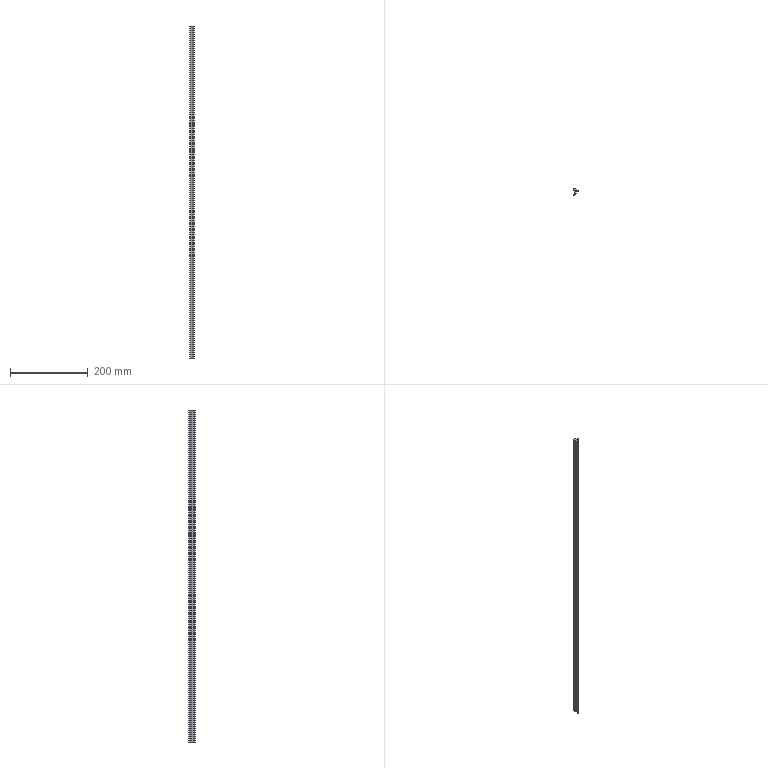Part | SolidWorks | features BaseBody 1, MoveFace 1 | 1 solid | 20 faces | box 10.8 x 17.5 x 856 mm | volume 67453 mm3 | cylinder 11 | plane 9 | commonest cylinder face diameters 1.6 x2 14 x2 0.4 x1 0.6 x1 0.8 x1 2.6 x1
STEP:
#1=CARTESIAN_POINT('',(-3.236,-11.055,756.));
#2=VERTEX_POINT('',#1);
#3=CARTESIAN_POINT('',(-4.3,-10.3,756.));
#4=VERTEX_POINT('',#3);
#5=CARTESIAN_POINT('',(-3.5,-10.3,756.));
#6=DIRECTION('',(0.,0.,-1.));
#7=DIRECTION('',(1.,0.,0.));
#8=AXIS2_PLACEMENT_3D('',#5,#6,#7);
#9=CIRCLE('',#8,0.8);
#10=EDGE_CURVE('',#2,#4,#9,.T.);
#11=ORIENTED_EDGE('',*,*,#10,.T.);
#12=CARTESIAN_POINT('',(-4.3,-10.3,-100.));
#13=VERTEX_POINT('',#12);
#14=CARTESIAN_POINT('',(-4.3,-10.3,-100.));
#15=DIRECTION('',(0.,0.,-1.));
#16=VECTOR('',#15,1000.);
#17=LINE('',#14,#16);
#18=EDGE_CURVE('',#4,#13,#17,.T.);
#19=ORIENTED_EDGE('',*,*,#18,.T.);
#20=CARTESIAN_POINT('',(-3.236,-11.055,-100.));
#21=VERTEX_POINT('',#20);
#22=CARTESIAN_POINT('',(-3.5,-10.3,-100.));
#23=DIRECTION('',(0.,0.,1.));
#24=DIRECTION('',(-1.,0.,0.));
#25=AXIS2_PLACEMENT_3D('',#22,#23,#24);
#26=CIRCLE('',#25,0.8);
#27=EDGE_CURVE('',#13,#21,#26,.T.);
#28=ORIENTED_EDGE('',*,*,#27,.T.);
#29=CARTESIAN_POINT('',(-3.236,-11.055,-100.));
#30=DIRECTION('',(0.,0.,-1.));
#31=VECTOR('',#30,1000.);
#32=LINE('',#29,#31);
#33=EDGE_CURVE('',#2,#21,#32,.T.);
#34=ORIENTED_EDGE('',*,*,#33,.F.);
#35=EDGE_LOOP('',(#11,#19,#28,#34));
#36=FACE_OUTER_BOUND('',#35,.T.);
#37=CARTESIAN_POINT('',(-3.5,-10.3,-100.));
#38=DIRECTION('',(0.,0.,-1.));
#39=DIRECTION('',(-1.,0.,0.));
#40=AXIS2_PLACEMENT_3D('',#37,#38,#39);
#41=CYLINDRICAL_SURFACE('',#40,0.8);
#42=ADVANCED_FACE('',(#36),#41,.T.);
#43=CARTESIAN_POINT('',(1.184,-6.397,-100.));
#44=VERTEX_POINT('',#43);
#45=CARTESIAN_POINT('',(-5.702,-4.29,-100.));
#46=DIRECTION('',(0.,0.,1.));
#47=DIRECTION('',(-1.,0.,0.));
#48=AXIS2_PLACEMENT_3D('',#45,#46,#47);
#49=CIRCLE('',#48,7.201);
#50=EDGE_CURVE('',#21,#44,#49,.T.);
#51=ORIENTED_EDGE('',*,*,#50,.T.);
#52=CARTESIAN_POINT('',(1.184,-6.397,756.));
#53=VERTEX_POINT('',#52);
#54=CARTESIAN_POINT('',(1.184,-6.397,-100.));
#55=DIRECTION('',(0.,0.,1.));
#56=VECTOR('',#55,1000.);
#57=LINE('',#54,#56);
#58=EDGE_CURVE('',#44,#53,#57,.T.);
#59=ORIENTED_EDGE('',*,*,#58,.T.);
#60=CARTESIAN_POINT('',(-5.702,-4.29,756.));
#61=DIRECTION('',(0.,0.,-1.));
#62=DIRECTION('',(1.,0.,0.));
#63=AXIS2_PLACEMENT_3D('',#60,#61,#62);
#64=CIRCLE('',#63,7.201);
#65=EDGE_CURVE('',#53,#2,#64,.T.);
#66=ORIENTED_EDGE('',*,*,#65,.T.);
#67=ORIENTED_EDGE('',*,*,#33,.T.);
#68=EDGE_LOOP('',(#51,#59,#66,#67));
#69=FACE_OUTER_BOUND('',#68,.T.);
#70=CARTESIAN_POINT('',(-5.702,-4.29,-100.));
#71=DIRECTION('',(0.,0.,-1.));
#72=DIRECTION('',(-1.,0.,0.));
#73=AXIS2_PLACEMENT_3D('',#70,#71,#72);
#74=CYLINDRICAL_SURFACE('',#73,7.201);
#75=ADVANCED_FACE('',(#69),#74,.T.);
#76=CARTESIAN_POINT('',(0.9,-6.,-100.));
#77=VERTEX_POINT('',#76);
#78=CARTESIAN_POINT('',(0.9,-6.3,-100.));
#79=DIRECTION('',(0.,0.,1.));
#80=DIRECTION('',(-1.,0.,0.));
#81=AXIS2_PLACEMENT_3D('',#78,#79,#80);
#82=CIRCLE('',#81,0.3);
#83=EDGE_CURVE('',#44,#77,#82,.T.);
#84=ORIENTED_EDGE('',*,*,#83,.T.);
#85=CARTESIAN_POINT('',(0.9,-6.,756.));
#86=VERTEX_POINT('',#85);
#87=CARTESIAN_POINT('',(0.9,-6.,-100.));
#88=DIRECTION('',(0.,0.,1.));
#89=VECTOR('',#88,1000.);
#90=LINE('',#87,#89);
#91=EDGE_CURVE('',#77,#86,#90,.T.);
#92=ORIENTED_EDGE('',*,*,#91,.T.);
#93=CARTESIAN_POINT('',(0.9,-6.3,756.));
#94=DIRECTION('',(0.,0.,-1.));
#95=DIRECTION('',(1.,0.,0.));
#96=AXIS2_PLACEMENT_3D('',#93,#94,#95);
#97=CIRCLE('',#96,0.3);
#98=EDGE_CURVE('',#86,#53,#97,.T.);
#99=ORIENTED_EDGE('',*,*,#98,.T.);
#100=ORIENTED_EDGE('',*,*,#58,.F.);
#101=EDGE_LOOP('',(#84,#92,#99,#100));
#102=FACE_OUTER_BOUND('',#101,.T.);
#103=CARTESIAN_POINT('',(0.9,-6.3,-100.));
#104=DIRECTION('',(0.,0.,-1.));
#105=DIRECTION('',(-1.,0.,0.));
#106=AXIS2_PLACEMENT_3D('',#103,#104,#105);
#107=CYLINDRICAL_SURFACE('',#106,0.3);
#108=ADVANCED_FACE('',(#102),#107,.T.);
#109=CARTESIAN_POINT('',(-2.5,-0.5,-100.));
#110=VERTEX_POINT('',#109);
#111=CARTESIAN_POINT('',(-2.5,-6.153,-100.));
#112=VERTEX_POINT('',#111);
#113=CARTESIAN_POINT('',(-2.5,-6.397,-100.));
#114=DIRECTION('',(0.,-1.,0.));
#115=VECTOR('',#114,1000.);
#116=LINE('',#113,#115);
#117=EDGE_CURVE('',#110,#112,#116,.T.);
#118=ORIENTED_EDGE('',*,*,#117,.F.);
#119=CARTESIAN_POINT('',(-4.2,1.695,-100.));
#120=VERTEX_POINT('',#119);
#121=CARTESIAN_POINT('',(-1.701,1.875,-100.));
#122=DIRECTION('',(0.,0.,1.));
#123=DIRECTION('',(-1.,0.,0.));
#124=AXIS2_PLACEMENT_3D('',#121,#122,#123);
#125=CIRCLE('',#124,2.506);
#126=EDGE_CURVE('',#120,#110,#125,.T.);
#127=ORIENTED_EDGE('',*,*,#126,.F.);
#128=CARTESIAN_POINT('',(-4.2,5.1,-100.));
#129=VERTEX_POINT('',#128);
#130=CARTESIAN_POINT('',(-4.2,-6.397,-100.));
#131=DIRECTION('',(0.,-1.,0.));
#132=VECTOR('',#131,1000.);
#133=LINE('',#130,#132);
#134=EDGE_CURVE('',#129,#120,#133,.T.);
#135=ORIENTED_EDGE('',*,*,#134,.F.);
#136=CARTESIAN_POINT('',(-2.892,6.4,-100.));
#137=VERTEX_POINT('',#136);
#138=CARTESIAN_POINT('',(-2.9,5.1,-100.));
#139=DIRECTION('',(0.,0.,1.));
#140=DIRECTION('',(-1.,0.,0.));
#141=AXIS2_PLACEMENT_3D('',#138,#139,#140);
#142=CIRCLE('',#141,1.3);
#143=EDGE_CURVE('',#137,#129,#142,.T.);
#144=ORIENTED_EDGE('',*,*,#143,.F.);
#145=CARTESIAN_POINT('',(0.5,5.5,-100.));
#146=VERTEX_POINT('',#145);
#147=CARTESIAN_POINT('',(-2.934,-0.5999,-100.));
#148=DIRECTION('',(0.,0.,1.));
#149=DIRECTION('',(-1.,0.,0.));
#150=AXIS2_PLACEMENT_3D('',#147,#148,#149);
#151=CIRCLE('',#150,7.);
#152=EDGE_CURVE('',#146,#137,#151,.T.);
#153=ORIENTED_EDGE('',*,*,#152,.F.);
#154=CARTESIAN_POINT('',(5.5,1.7,-100.));
#155=VERTEX_POINT('',#154);
#156=CARTESIAN_POINT('',(5.5,1.7,-100.));
#157=DIRECTION('',(-0.7962,0.6051,0.));
#158=VECTOR('',#157,1000.);
#159=LINE('',#156,#158);
#160=EDGE_CURVE('',#155,#146,#159,.T.);
#161=ORIENTED_EDGE('',*,*,#160,.F.);
#162=CARTESIAN_POINT('',(6.458,-0.2215,-100.));
#163=VERTEX_POINT('',#162);
#164=CARTESIAN_POINT('',(6.458,-0.2215,-100.));
#165=DIRECTION('',(-0.4462,0.8949,0.));
#166=VECTOR('',#165,1000.);
#167=LINE('',#164,#166);
#168=EDGE_CURVE('',#163,#155,#167,.T.);
#169=ORIENTED_EDGE('',*,*,#168,.F.);
#170=CARTESIAN_POINT('',(5.895,-0.7433,-100.));
#171=VERTEX_POINT('',#170);
#172=CARTESIAN_POINT('',(6.1,-0.4,-100.));
#173=DIRECTION('',(0.,0.,1.));
#174=DIRECTION('',(-1.,0.,0.));
#175=AXIS2_PLACEMENT_3D('',#172,#173,#174);
#176=CIRCLE('',#175,0.4);
#177=EDGE_CURVE('',#171,#163,#176,.T.);
#178=ORIENTED_EDGE('',*,*,#177,.F.);
#179=CARTESIAN_POINT('',(3.,0.,-100.));
#180=VERTEX_POINT('',#179);
#181=CARTESIAN_POINT('',(2.746,-6.995,-100.));
#182=DIRECTION('',(0.,0.,-1.));
#183=DIRECTION('',(-1.,0.,0.));
#184=AXIS2_PLACEMENT_3D('',#181,#182,#183);
#185=CIRCLE('',#184,7.);
#186=EDGE_CURVE('',#180,#171,#185,.T.);
#187=ORIENTED_EDGE('',*,*,#186,.F.);
#188=CARTESIAN_POINT('',(0.,0.,-100.));
#189=VERTEX_POINT('',#188);
#190=CARTESIAN_POINT('',(-6.814,0.,-100.));
#191=DIRECTION('',(1.,0.,0.));
#192=VECTOR('',#191,1000.);
#193=LINE('',#190,#192);
#194=EDGE_CURVE('',#189,#180,#193,.T.);
#195=ORIENTED_EDGE('',*,*,#194,.F.);
#196=CARTESIAN_POINT('',(0.,-5.8,-100.));
#197=VERTEX_POINT('',#196);
#198=CARTESIAN_POINT('',(0.,-6.397,-100.));
#199=DIRECTION('',(0.,1.,0.));
#200=VECTOR('',#199,1000.);
#201=LINE('',#198,#200);
#202=EDGE_CURVE('',#197,#189,#201,.T.);
#203=ORIENTED_EDGE('',*,*,#202,.F.);
#204=CARTESIAN_POINT('',(0.2,-6.,-100.));
#205=VERTEX_POINT('',#204);
#206=CARTESIAN_POINT('',(0.2,-5.8,-100.));
#207=DIRECTION('',(0.,0.,1.));
#208=DIRECTION('',(-1.,0.,0.));
#209=AXIS2_PLACEMENT_3D('',#206,#207,#208);
#210=CIRCLE('',#209,0.2);
#211=EDGE_CURVE('',#197,#205,#210,.T.);
#212=ORIENTED_EDGE('',*,*,#211,.T.);
#213=CARTESIAN_POINT('',(-6.814,-6.,-100.));
#214=DIRECTION('',(-1.,0.,0.));
#215=VECTOR('',#214,1000.);
#216=LINE('',#213,#215);
#217=EDGE_CURVE('',#77,#205,#216,.T.);
#218=ORIENTED_EDGE('',*,*,#217,.F.);
#219=ORIENTED_EDGE('',*,*,#83,.F.);
#220=ORIENTED_EDGE('',*,*,#50,.F.);
#221=ORIENTED_EDGE('',*,*,#27,.F.);
#222=CARTESIAN_POINT('',(-3.998,-9.674,-100.));
#223=VERTEX_POINT('',#222);
#224=CARTESIAN_POINT('',(-3.5,-10.3,-100.));
#225=DIRECTION('',(0.,0.,1.));
#226=DIRECTION('',(-1.,0.,0.));
#227=AXIS2_PLACEMENT_3D('',#224,#225,#226);
#228=CIRCLE('',#227,0.8);
#229=EDGE_CURVE('',#223,#13,#228,.T.);
#230=ORIENTED_EDGE('',*,*,#229,.F.);
#231=CARTESIAN_POINT('',(-6.814,-6.397,-100.));
#232=DIRECTION('',(0.,0.,-1.));
#233=DIRECTION('',(-1.,0.,0.));
#234=AXIS2_PLACEMENT_3D('',#231,#232,#233);
#235=CIRCLE('',#234,4.321);
#236=EDGE_CURVE('',#112,#223,#235,.T.);
#237=ORIENTED_EDGE('',*,*,#236,.F.);
#238=EDGE_LOOP('',(#118,#127,#135,#144,#153,#161,#169,#178,#187,#195,#203,#212,#218,#219,#220,#221,#230,#237));
#239=FACE_OUTER_BOUND('',#238,.T.);
#240=CARTESIAN_POINT('',(-6.814,-6.397,-100.));
#241=DIRECTION('',(0.,0.,1.));
#242=DIRECTION('',(1.,0.,0.));
#243=AXIS2_PLACEMENT_3D('',#240,#241,#242);
#244=PLANE('',#243);
#245=ADVANCED_FACE('',(#239),#244,.F.);
#246=ORIENTED_EDGE('',*,*,#18,.F.);
#247=CARTESIAN_POINT('',(-3.998,-9.674,756.));
#248=VERTEX_POINT('',#247);
#249=CARTESIAN_POINT('',(-3.5,-10.3,756.));
#250=DIRECTION('',(0.,0.,-1.));
#251=DIRECTION('',(1.,0.,0.));
#252=AXIS2_PLACEMENT_3D('',#249,#250,#251);
#253=CIRCLE('',#252,0.8);
#254=EDGE_CURVE('',#4,#248,#253,.T.);
#255=ORIENTED_EDGE('',*,*,#254,.T.);
#256=CARTESIAN_POINT('',(-3.998,-9.674,-100.));
#257=DIRECTION('',(0.,0.,-1.));
#258=VECTOR('',#257,1000.);
#259=LINE('',#256,#258);
#260=EDGE_CURVE('',#248,#223,#259,.T.);
#261=ORIENTED_EDGE('',*,*,#260,.T.);
#262=ORIENTED_EDGE('',*,*,#229,.T.);
#263=EDGE_LOOP('',(#246,#255,#261,#262));
#264=FACE_OUTER_BOUND('',#263,.T.);
#265=CARTESIAN_POINT('',(-3.5,-10.3,-100.));
#266=DIRECTION('',(0.,0.,-1.));
#267=DIRECTION('',(-1.,0.,0.));
#268=AXIS2_PLACEMENT_3D('',#265,#266,#267);
#269=CYLINDRICAL_SURFACE('',#268,0.8);
#270=ADVANCED_FACE('',(#264),#269,.T.);
#271=CARTESIAN_POINT('',(-4.2,1.695,756.));
#272=VERTEX_POINT('',#271);
#273=CARTESIAN_POINT('',(-2.5,-0.5,756.));
#274=VERTEX_POINT('',#273);
#275=CARTESIAN_POINT('',(-1.701,1.875,756.));
#276=DIRECTION('',(0.,0.,1.));
#277=DIRECTION('',(1.,0.,0.));
#278=AXIS2_PLACEMENT_3D('',#275,#276,#277);
#279=CIRCLE('',#278,2.506);
#280=EDGE_CURVE('',#272,#274,#279,.T.);
#281=ORIENTED_EDGE('',*,*,#280,.T.);
#282=CARTESIAN_POINT('',(-2.5,-6.153,756.));
#283=VERTEX_POINT('',#282);
#284=CARTESIAN_POINT('',(-2.5,-6.397,756.));
#285=DIRECTION('',(0.,-1.,0.));
#286=VECTOR('',#285,1000.);
#287=LINE('',#284,#286);
#288=EDGE_CURVE('',#274,#283,#287,.T.);
#289=ORIENTED_EDGE('',*,*,#288,.T.);
#290=CARTESIAN_POINT('',(-6.814,-6.397,756.));
#291=DIRECTION('',(0.,0.,-1.));
#292=DIRECTION('',(1.,0.,0.));
#293=AXIS2_PLACEMENT_3D('',#290,#291,#292);
#294=CIRCLE('',#293,4.321);
#295=EDGE_CURVE('',#283,#248,#294,.T.);
#296=ORIENTED_EDGE('',*,*,#295,.T.);
#297=ORIENTED_EDGE('',*,*,#254,.F.);
#298=ORIENTED_EDGE('',*,*,#10,.F.);
#299=ORIENTED_EDGE('',*,*,#65,.F.);
#300=ORIENTED_EDGE('',*,*,#98,.F.);
#301=CARTESIAN_POINT('',(0.2,-6.,756.));
#302=VERTEX_POINT('',#301);
#303=CARTESIAN_POINT('',(-6.814,-6.,756.));
#304=DIRECTION('',(-1.,0.,0.));
#305=VECTOR('',#304,1000.);
#306=LINE('',#303,#305);
#307=EDGE_CURVE('',#86,#302,#306,.T.);
#308=ORIENTED_EDGE('',*,*,#307,.T.);
#309=CARTESIAN_POINT('',(0.,-5.8,756.));
#310=VERTEX_POINT('',#309);
#311=CARTESIAN_POINT('',(0.2,-5.8,756.));
#312=DIRECTION('',(0.,0.,-1.));
#313=DIRECTION('',(1.,0.,0.));
#314=AXIS2_PLACEMENT_3D('',#311,#312,#313);
#315=CIRCLE('',#314,0.2);
#316=EDGE_CURVE('',#302,#310,#315,.T.);
#317=ORIENTED_EDGE('',*,*,#316,.T.);
#318=CARTESIAN_POINT('',(0.,0.,756.));
#319=VERTEX_POINT('',#318);
#320=CARTESIAN_POINT('',(0.,-6.397,756.));
#321=DIRECTION('',(0.,1.,0.));
#322=VECTOR('',#321,1000.);
#323=LINE('',#320,#322);
#324=EDGE_CURVE('',#310,#319,#323,.T.);
#325=ORIENTED_EDGE('',*,*,#324,.T.);
#326=CARTESIAN_POINT('',(3.,0.,756.));
#327=VERTEX_POINT('',#326);
#328=CARTESIAN_POINT('',(-6.814,0.,756.));
#329=DIRECTION('',(1.,0.,0.));
#330=VECTOR('',#329,1000.);
#331=LINE('',#328,#330);
#332=EDGE_CURVE('',#319,#327,#331,.T.);
#333=ORIENTED_EDGE('',*,*,#332,.T.);
#334=CARTESIAN_POINT('',(5.895,-0.7433,756.));
#335=VERTEX_POINT('',#334);
#336=CARTESIAN_POINT('',(2.746,-6.995,756.));
#337=DIRECTION('',(0.,0.,-1.));
#338=DIRECTION('',(1.,0.,0.));
#339=AXIS2_PLACEMENT_3D('',#336,#337,#338);
#340=CIRCLE('',#339,7.);
#341=EDGE_CURVE('',#327,#335,#340,.T.);
#342=ORIENTED_EDGE('',*,*,#341,.T.);
#343=CARTESIAN_POINT('',(6.458,-0.2215,756.));
#344=VERTEX_POINT('',#343);
#345=CARTESIAN_POINT('',(6.1,-0.4,756.));
#346=DIRECTION('',(0.,0.,-1.));
#347=DIRECTION('',(1.,0.,0.));
#348=AXIS2_PLACEMENT_3D('',#345,#346,#347);
#349=CIRCLE('',#348,0.4);
#350=EDGE_CURVE('',#344,#335,#349,.T.);
#351=ORIENTED_EDGE('',*,*,#350,.F.);
#352=CARTESIAN_POINT('',(5.5,1.7,756.));
#353=VERTEX_POINT('',#352);
#354=CARTESIAN_POINT('',(6.282,0.1323,756.));
#355=DIRECTION('',(-0.4462,0.8949,0.));
#356=VECTOR('',#355,1000.);
#357=LINE('',#354,#356);
#358=EDGE_CURVE('',#344,#353,#357,.T.);
#359=ORIENTED_EDGE('',*,*,#358,.T.);
#360=CARTESIAN_POINT('',(0.5,5.5,756.));
#361=VERTEX_POINT('',#360);
#362=CARTESIAN_POINT('',(1.595,4.668,756.));
#363=DIRECTION('',(-0.7962,0.6051,0.));
#364=VECTOR('',#363,1000.);
#365=LINE('',#362,#364);
#366=EDGE_CURVE('',#353,#361,#365,.T.);
#367=ORIENTED_EDGE('',*,*,#366,.T.);
#368=CARTESIAN_POINT('',(-2.892,6.4,756.));
#369=VERTEX_POINT('',#368);
#370=CARTESIAN_POINT('',(-2.934,-0.5999,756.));
#371=DIRECTION('',(0.,0.,1.));
#372=DIRECTION('',(1.,0.,0.));
#373=AXIS2_PLACEMENT_3D('',#370,#371,#372);
#374=CIRCLE('',#373,7.);
#375=EDGE_CURVE('',#361,#369,#374,.T.);
#376=ORIENTED_EDGE('',*,*,#375,.T.);
#377=CARTESIAN_POINT('',(-4.2,5.1,756.));
#378=VERTEX_POINT('',#377);
#379=CARTESIAN_POINT('',(-2.9,5.1,756.));
#380=DIRECTION('',(0.,0.,1.));
#381=DIRECTION('',(1.,0.,0.));
#382=AXIS2_PLACEMENT_3D('',#379,#380,#381);
#383=CIRCLE('',#382,1.3);
#384=EDGE_CURVE('',#369,#378,#383,.T.);
#385=ORIENTED_EDGE('',*,*,#384,.T.);
#386=CARTESIAN_POINT('',(-4.2,-6.397,756.));
#387=DIRECTION('',(0.,-1.,0.));
#388=VECTOR('',#387,1000.);
#389=LINE('',#386,#388);
#390=EDGE_CURVE('',#378,#272,#389,.T.);
#391=ORIENTED_EDGE('',*,*,#390,.T.);
#392=EDGE_LOOP('',(#281,#289,#296,#297,#298,#299,#300,#308,#317,#325,#333,#342,#351,#359,#367,#376,#385,#391));
#393=FACE_OUTER_BOUND('',#392,.T.);
#394=CARTESIAN_POINT('',(-6.814,-6.397,756.));
#395=DIRECTION('',(0.,0.,1.));
#396=DIRECTION('',(1.,0.,0.));
#397=AXIS2_PLACEMENT_3D('',#394,#395,#396);
#398=PLANE('',#397);
#399=ADVANCED_FACE('',(#393),#398,.T.);
#400=ORIENTED_EDGE('',*,*,#217,.T.);
#401=CARTESIAN_POINT('',(0.2,-6.,-100.));
#402=DIRECTION('',(0.,0.,1.));
#403=VECTOR('',#402,1000.);
#404=LINE('',#401,#403);
#405=EDGE_CURVE('',#205,#302,#404,.T.);
#406=ORIENTED_EDGE('',*,*,#405,.T.);
#407=ORIENTED_EDGE('',*,*,#307,.F.);
#408=ORIENTED_EDGE('',*,*,#91,.F.);
#409=EDGE_LOOP('',(#400,#406,#407,#408));
#410=FACE_OUTER_BOUND('',#409,.T.);
#411=CARTESIAN_POINT('',(0.9,-6.,-100.));
#412=DIRECTION('',(0.,1.,0.));
#413=DIRECTION('',(0.,0.,1.));
#414=AXIS2_PLACEMENT_3D('',#411,#412,#413);
#415=PLANE('',#414);
#416=ADVANCED_FACE('',(#410),#415,.T.);
#417=CARTESIAN_POINT('',(-2.5,-6.153,-100.));
#418=DIRECTION('',(0.,0.,1.));
#419=VECTOR('',#418,1000.);
#420=LINE('',#417,#419);
#421=EDGE_CURVE('',#112,#283,#420,.T.);
#422=ORIENTED_EDGE('',*,*,#421,.F.);
#423=ORIENTED_EDGE('',*,*,#236,.T.);
#424=ORIENTED_EDGE('',*,*,#260,.F.);
#425=ORIENTED_EDGE('',*,*,#295,.F.);
#426=EDGE_LOOP('',(#422,#423,#424,#425));
#427=FACE_OUTER_BOUND('',#426,.T.);
#428=CARTESIAN_POINT('',(-6.814,-6.397,-100.));
#429=DIRECTION('',(0.,0.,-1.));
#430=DIRECTION('',(-1.,0.,0.));
#431=AXIS2_PLACEMENT_3D('',#428,#429,#430);
#432=CYLINDRICAL_SURFACE('',#431,4.321);
#433=ADVANCED_FACE('',(#427),#432,.F.);
#434=ORIENTED_EDGE('',*,*,#117,.T.);
#435=ORIENTED_EDGE('',*,*,#421,.T.);
#436=ORIENTED_EDGE('',*,*,#288,.F.);
#437=CARTESIAN_POINT('',(-2.5,-0.5,-100.));
#438=DIRECTION('',(0.,0.,-1.));
#439=VECTOR('',#438,1000.);
#440=LINE('',#437,#439);
#441=EDGE_CURVE('',#274,#110,#440,.T.);
#442=ORIENTED_EDGE('',*,*,#441,.T.);
#443=EDGE_LOOP('',(#434,#435,#436,#442));
#444=FACE_OUTER_BOUND('',#443,.T.);
#445=CARTESIAN_POINT('',(-2.5,-0.5,-100.));
#446=DIRECTION('',(-1.,0.,0.));
#447=DIRECTION('',(0.,0.,1.));
#448=AXIS2_PLACEMENT_3D('',#445,#446,#447);
#449=PLANE('',#448);
#450=ADVANCED_FACE('',(#444),#449,.T.);
#451=ORIENTED_EDGE('',*,*,#126,.T.);
#452=ORIENTED_EDGE('',*,*,#441,.F.);
#453=ORIENTED_EDGE('',*,*,#280,.F.);
#454=CARTESIAN_POINT('',(-4.2,1.695,-100.));
#455=DIRECTION('',(0.,0.,-1.));
#456=VECTOR('',#455,1000.);
#457=LINE('',#454,#456);
#458=EDGE_CURVE('',#272,#120,#457,.T.);
#459=ORIENTED_EDGE('',*,*,#458,.T.);
#460=EDGE_LOOP('',(#451,#452,#453,#459));
#461=FACE_OUTER_BOUND('',#460,.T.);
#462=CARTESIAN_POINT('',(-1.701,1.875,-100.));
#463=DIRECTION('',(0.,0.,-1.));
#464=DIRECTION('',(-1.,0.,0.));
#465=AXIS2_PLACEMENT_3D('',#462,#463,#464);
#466=CYLINDRICAL_SURFACE('',#465,2.506);
#467=ADVANCED_FACE('',(#461),#466,.T.);
#468=ORIENTED_EDGE('',*,*,#134,.T.);
#469=ORIENTED_EDGE('',*,*,#458,.F.);
#470=ORIENTED_EDGE('',*,*,#390,.F.);
#471=CARTESIAN_POINT('',(-4.2,5.1,-100.));
#472=DIRECTION('',(0.,0.,-1.));
#473=VECTOR('',#472,1000.);
#474=LINE('',#471,#473);
#475=EDGE_CURVE('',#378,#129,#474,.T.);
#476=ORIENTED_EDGE('',*,*,#475,.T.);
#477=EDGE_LOOP('',(#468,#469,#470,#476));
#478=FACE_OUTER_BOUND('',#477,.T.);
#479=CARTESIAN_POINT('',(-4.2,5.1,-100.));
#480=DIRECTION('',(-1.,0.,0.));
#481=DIRECTION('',(0.,0.,1.));
#482=AXIS2_PLACEMENT_3D('',#479,#480,#481);
#483=PLANE('',#482);
#484=ADVANCED_FACE('',(#478),#483,.T.);
#485=ORIENTED_EDGE('',*,*,#143,.T.);
#486=ORIENTED_EDGE('',*,*,#475,.F.);
#487=ORIENTED_EDGE('',*,*,#384,.F.);
#488=CARTESIAN_POINT('',(-2.892,6.4,-100.));
#489=DIRECTION('',(0.,0.,-1.));
#490=VECTOR('',#489,1000.);
#491=LINE('',#488,#490);
#492=EDGE_CURVE('',#369,#137,#491,.T.);
#493=ORIENTED_EDGE('',*,*,#492,.T.);
#494=EDGE_LOOP('',(#485,#486,#487,#493));
#495=FACE_OUTER_BOUND('',#494,.T.);
#496=CARTESIAN_POINT('',(-2.9,5.1,-100.));
#497=DIRECTION('',(0.,0.,-1.));
#498=DIRECTION('',(-1.,0.,0.));
#499=AXIS2_PLACEMENT_3D('',#496,#497,#498);
#500=CYLINDRICAL_SURFACE('',#499,1.3);
#501=ADVANCED_FACE('',(#495),#500,.T.);
#502=ORIENTED_EDGE('',*,*,#152,.T.);
#503=ORIENTED_EDGE('',*,*,#492,.F.);
#504=ORIENTED_EDGE('',*,*,#375,.F.);
#505=CARTESIAN_POINT('',(0.5,5.5,-100.));
#506=DIRECTION('',(0.,0.,-1.));
#507=VECTOR('',#506,1000.);
#508=LINE('',#505,#507);
#509=EDGE_CURVE('',#361,#146,#508,.T.);
#510=ORIENTED_EDGE('',*,*,#509,.T.);
#511=EDGE_LOOP('',(#502,#503,#504,#510));
#512=FACE_OUTER_BOUND('',#511,.T.);
#513=CARTESIAN_POINT('',(-2.934,-0.5999,-100.));
#514=DIRECTION('',(0.,0.,-1.));
#515=DIRECTION('',(-1.,0.,0.));
#516=AXIS2_PLACEMENT_3D('',#513,#514,#515);
#517=CYLINDRICAL_SURFACE('',#516,7.);
#518=ADVANCED_FACE('',(#512),#517,.T.);
#519=ORIENTED_EDGE('',*,*,#160,.T.);
#520=ORIENTED_EDGE('',*,*,#509,.F.);
#521=ORIENTED_EDGE('',*,*,#366,.F.);
#522=CARTESIAN_POINT('',(5.5,1.7,-100.));
#523=DIRECTION('',(0.,0.,-1.));
#524=VECTOR('',#523,1000.);
#525=LINE('',#522,#524);
#526=EDGE_CURVE('',#353,#155,#525,.T.);
#527=ORIENTED_EDGE('',*,*,#526,.T.);
#528=EDGE_LOOP('',(#519,#520,#521,#527));
#529=FACE_OUTER_BOUND('',#528,.T.);
#530=CARTESIAN_POINT('',(5.5,1.7,-100.));
#531=DIRECTION('',(0.6051,0.7962,0.));
#532=DIRECTION('',(-0.7962,0.6051,0.));
#533=AXIS2_PLACEMENT_3D('',#530,#531,#532);
#534=PLANE('',#533);
#535=ADVANCED_FACE('',(#529),#534,.T.);
#536=ORIENTED_EDGE('',*,*,#168,.T.);
#537=ORIENTED_EDGE('',*,*,#526,.F.);
#538=ORIENTED_EDGE('',*,*,#358,.F.);
#539=CARTESIAN_POINT('',(6.458,-0.2215,-100.));
#540=DIRECTION('',(0.,0.,-1.));
#541=VECTOR('',#540,1000.);
#542=LINE('',#539,#541);
#543=EDGE_CURVE('',#344,#163,#542,.T.);
#544=ORIENTED_EDGE('',*,*,#543,.T.);
#545=EDGE_LOOP('',(#536,#537,#538,#544));
#546=FACE_OUTER_BOUND('',#545,.T.);
#547=CARTESIAN_POINT('',(6.458,-0.2215,-100.));
#548=DIRECTION('',(0.8949,0.4462,0.));
#549=DIRECTION('',(-0.4462,0.8949,0.));
#550=AXIS2_PLACEMENT_3D('',#547,#548,#549);
#551=PLANE('',#550);
#552=ADVANCED_FACE('',(#546),#551,.T.);
#553=CARTESIAN_POINT('',(3.,0.,-100.));
#554=DIRECTION('',(0.,0.,1.));
#555=VECTOR('',#554,1000.);
#556=LINE('',#553,#555);
#557=EDGE_CURVE('',#180,#327,#556,.T.);
#558=ORIENTED_EDGE('',*,*,#557,.F.);
#559=ORIENTED_EDGE('',*,*,#186,.T.);
#560=CARTESIAN_POINT('',(5.895,-0.7433,-100.));
#561=DIRECTION('',(0.,0.,-1.));
#562=VECTOR('',#561,1000.);
#563=LINE('',#560,#562);
#564=EDGE_CURVE('',#335,#171,#563,.T.);
#565=ORIENTED_EDGE('',*,*,#564,.F.);
#566=ORIENTED_EDGE('',*,*,#341,.F.);
#567=EDGE_LOOP('',(#558,#559,#565,#566));
#568=FACE_OUTER_BOUND('',#567,.T.);
#569=CARTESIAN_POINT('',(2.746,-6.995,-100.));
#570=DIRECTION('',(0.,0.,-1.));
#571=DIRECTION('',(-1.,0.,0.));
#572=AXIS2_PLACEMENT_3D('',#569,#570,#571);
#573=CYLINDRICAL_SURFACE('',#572,7.);
#574=ADVANCED_FACE('',(#568),#573,.F.);
#575=ORIENTED_EDGE('',*,*,#194,.T.);
#576=ORIENTED_EDGE('',*,*,#557,.T.);
#577=ORIENTED_EDGE('',*,*,#332,.F.);
#578=CARTESIAN_POINT('',(0.,0.,-100.));
#579=DIRECTION('',(0.,0.,-1.));
#580=VECTOR('',#579,1000.);
#581=LINE('',#578,#580);
#582=EDGE_CURVE('',#319,#189,#581,.T.);
#583=ORIENTED_EDGE('',*,*,#582,.T.);
#584=EDGE_LOOP('',(#575,#576,#577,#583));
#585=FACE_OUTER_BOUND('',#584,.T.);
#586=CARTESIAN_POINT('',(0.,0.,-100.));
#587=DIRECTION('',(0.,-1.,0.));
#588=DIRECTION('',(0.,0.,-1.));
#589=AXIS2_PLACEMENT_3D('',#586,#587,#588);
#590=PLANE('',#589);
#591=ADVANCED_FACE('',(#585),#590,.T.);
#592=ORIENTED_EDGE('',*,*,#202,.T.);
#593=ORIENTED_EDGE('',*,*,#582,.F.);
#594=ORIENTED_EDGE('',*,*,#324,.F.);
#595=CARTESIAN_POINT('',(0.,-5.8,-100.));
#596=DIRECTION('',(0.,0.,-1.));
#597=VECTOR('',#596,1000.);
#598=LINE('',#595,#597);
#599=EDGE_CURVE('',#310,#197,#598,.T.);
#600=ORIENTED_EDGE('',*,*,#599,.T.);
#601=EDGE_LOOP('',(#592,#593,#594,#600));
#602=FACE_OUTER_BOUND('',#601,.T.);
#603=CARTESIAN_POINT('',(0.,-5.8,-100.));
#604=DIRECTION('',(1.,0.,0.));
#605=DIRECTION('',(0.,0.,-1.));
#606=AXIS2_PLACEMENT_3D('',#603,#604,#605);
#607=PLANE('',#606);
#608=ADVANCED_FACE('',(#602),#607,.T.);
#609=ORIENTED_EDGE('',*,*,#405,.F.);
#610=ORIENTED_EDGE('',*,*,#211,.F.);
#611=ORIENTED_EDGE('',*,*,#599,.F.);
#612=ORIENTED_EDGE('',*,*,#316,.F.);
#613=EDGE_LOOP('',(#609,#610,#611,#612));
#614=FACE_OUTER_BOUND('',#613,.T.);
#615=CARTESIAN_POINT('',(0.2,-5.8,-100.));
#616=DIRECTION('',(0.,0.,-1.));
#617=DIRECTION('',(-1.,0.,0.));
#618=AXIS2_PLACEMENT_3D('',#615,#616,#617);
#619=CYLINDRICAL_SURFACE('',#618,0.2);
#620=ADVANCED_FACE('',(#614),#619,.F.);
#621=ORIENTED_EDGE('',*,*,#177,.T.);
#622=ORIENTED_EDGE('',*,*,#543,.F.);
#623=ORIENTED_EDGE('',*,*,#350,.T.);
#624=ORIENTED_EDGE('',*,*,#564,.T.);
#625=EDGE_LOOP('',(#621,#622,#623,#624));
#626=FACE_OUTER_BOUND('',#625,.T.);
#627=CARTESIAN_POINT('',(6.1,-0.4,-100.));
#628=DIRECTION('',(0.,0.,-1.));
#629=DIRECTION('',(-1.,0.,0.));
#630=AXIS2_PLACEMENT_3D('',#627,#628,#629);
#631=CYLINDRICAL_SURFACE('',#630,0.4);
#632=ADVANCED_FACE('',(#626),#631,.T.);
#633=CLOSED_SHELL('',(#42,#75,#108,#245,#270,#399,#416,#433,#450,#467,#484,#501,#518,#535,#552,#574,#591,#608,#620,#632));
#634=MANIFOLD_SOLID_BREP('',#633);
#635=CARTESIAN_POINT('',(0.,0.,0.));
#636=DIRECTION('',(0.,0.,1.));
#637=DIRECTION('',(1.,0.,0.));
#638=AXIS2_PLACEMENT_3D('',#635,#636,#637);
#639=(LENGTH_UNIT()NAMED_UNIT(*)SI_UNIT(.MILLI.,.METRE.));
#640=UNCERTAINTY_MEASURE_WITH_UNIT(LENGTH_MEASURE(0.00001),#639,'','');
#641=(NAMED_UNIT(*)PLANE_ANGLE_UNIT()SI_UNIT($,.RADIAN.));
#642=(NAMED_UNIT(*)SI_UNIT($,.STERADIAN.)SOLID_ANGLE_UNIT());
#643=(GEOMETRIC_REPRESENTATION_CONTEXT(3)GLOBAL_UNCERTAINTY_ASSIGNED_CONTEXT((#640))GLOBAL_UNIT_ASSIGNED_CONTEXT((#639,#641,#642))REPRESENTATION_CONTEXT('',''));
#644=ADVANCED_BREP_SHAPE_REPRESENTATION('',(#634,#638),#643);